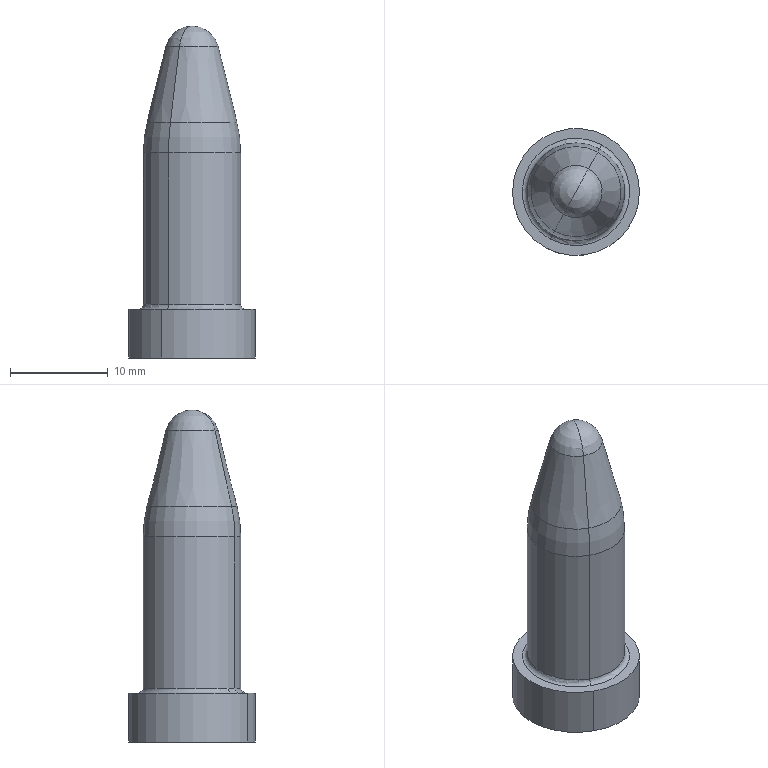Part | CATIA | 1 solid | 14 faces | box 13 x 13 x 34 mm | volume 2517 mm3 | cylinder 4 | torus 2 | other 2 | cone 2 | sphere 2 | plane 2 | commonest cylinder face diameters 10 x2 13 x2
STEP:
#1=CARTESIAN_POINT('',(3.116,5.704,-5.));
#2=VERTEX_POINT('',#1);
#3=CARTESIAN_POINT('',(-3.116,-5.704,-5.));
#4=VERTEX_POINT('',#3);
#5=CARTESIAN_POINT('',(0.,0.,-5.));
#6=DIRECTION('',(0.,0.,-1.));
#7=AXIS2_PLACEMENT_3D('',#5,#6,$);
#8=CIRCLE('',#7,6.5);
#9=EDGE_CURVE('',#2,#4,#8,.T.);
#10=ORIENTED_EDGE('',*,*,#9,.F.);
#11=CARTESIAN_POINT('',(3.116,5.704,0.));
#12=VERTEX_POINT('',#11);
#13=CARTESIAN_POINT('',(3.116,5.704,-2.5));
#14=DIRECTION('',(0.,0.,-1.));
#15=VECTOR('',#14,1.);
#16=LINE('',#13,#15);
#17=EDGE_CURVE('',#2,#12,#16,.F.);
#18=ORIENTED_EDGE('',*,*,#17,.T.);
#19=CARTESIAN_POINT('',(-3.116,-5.704,0.));
#20=VERTEX_POINT('',#19);
#21=CARTESIAN_POINT('',(0.,0.,0.));
#22=DIRECTION('',(0.,0.,-1.));
#23=AXIS2_PLACEMENT_3D('',#21,#22,$);
#24=CIRCLE('',#23,6.5);
#25=EDGE_CURVE('',#12,#20,#24,.T.);
#26=ORIENTED_EDGE('',*,*,#25,.T.);
#27=CARTESIAN_POINT('',(-3.116,-5.704,-2.5));
#28=DIRECTION('',(0.,0.,-1.));
#29=VECTOR('',#28,1.);
#30=LINE('',#27,#29);
#31=EDGE_CURVE('',#4,#20,#30,.F.);
#32=ORIENTED_EDGE('',*,*,#31,.F.);
#33=EDGE_LOOP('',(#10,#18,#26,#32));
#34=FACE_OUTER_BOUND('',#33,.T.);
#35=CARTESIAN_POINT('',(0.,0.,12.));
#36=DIRECTION('',(0.,0.,-1.));
#37=DIRECTION('',(0.4794,0.8776,0.));
#38=AXIS2_PLACEMENT_3D('',#35,#36,#37);
#39=CYLINDRICAL_SURFACE('',#38,6.5);
#40=ADVANCED_FACE('',(#34),#39,.T.);
#41=CARTESIAN_POINT('',(0.,0.,-5.));
#42=DIRECTION('',(0.,0.,-1.));
#43=AXIS2_PLACEMENT_3D('',#41,#42,$);
#44=CIRCLE('',#43,6.5);
#45=EDGE_CURVE('',#4,#2,#44,.T.);
#46=ORIENTED_EDGE('',*,*,#45,.F.);
#47=ORIENTED_EDGE('',*,*,#31,.T.);
#48=CARTESIAN_POINT('',(0.,0.,0.));
#49=DIRECTION('',(0.,0.,-1.));
#50=AXIS2_PLACEMENT_3D('',#48,#49,$);
#51=CIRCLE('',#50,6.5);
#52=EDGE_CURVE('',#20,#12,#51,.T.);
#53=ORIENTED_EDGE('',*,*,#52,.T.);
#54=ORIENTED_EDGE('',*,*,#17,.F.);
#55=EDGE_LOOP('',(#46,#47,#53,#54));
#56=FACE_OUTER_BOUND('',#55,.T.);
#57=ADVANCED_FACE('',(#56),#39,.T.);
#58=CARTESIAN_POINT('',(2.637,4.827,0.));
#59=VERTEX_POINT('',#58);
#60=CARTESIAN_POINT('',(-2.637,-4.827,0.));
#61=VERTEX_POINT('',#60);
#62=CARTESIAN_POINT('',(0.,0.,0.));
#63=DIRECTION('',(0.,0.,-1.));
#64=AXIS2_PLACEMENT_3D('',#62,#63,$);
#65=CIRCLE('',#64,5.5);
#66=EDGE_CURVE('',#59,#61,#65,.T.);
#67=ORIENTED_EDGE('',*,*,#66,.F.);
#68=CARTESIAN_POINT('',(2.397,4.388,0.5));
#69=VERTEX_POINT('',#68);
#70=CARTESIAN_POINT('',(2.637,4.827,0.5));
#71=DIRECTION('',(-0.8776,0.4794,0.));
#72=AXIS2_PLACEMENT_3D('',#70,#71,$);
#73=CIRCLE('',#72,0.5);
#74=EDGE_CURVE('',#59,#69,#73,.T.);
#75=ORIENTED_EDGE('',*,*,#74,.T.);
#76=CARTESIAN_POINT('',(-2.397,-4.388,0.5));
#77=VERTEX_POINT('',#76);
#78=CARTESIAN_POINT('',(0.,0.,0.5));
#79=DIRECTION('',(0.,0.,-1.));
#80=AXIS2_PLACEMENT_3D('',#78,#79,$);
#81=CIRCLE('',#80,5.);
#82=EDGE_CURVE('',#69,#77,#81,.T.);
#83=ORIENTED_EDGE('',*,*,#82,.T.);
#84=CARTESIAN_POINT('',(-2.637,-4.827,0.5));
#85=DIRECTION('',(0.8776,-0.4794,0.));
#86=AXIS2_PLACEMENT_3D('',#84,#85,$);
#87=CIRCLE('',#86,0.5);
#88=EDGE_CURVE('',#61,#77,#87,.T.);
#89=ORIENTED_EDGE('',*,*,#88,.F.);
#90=EDGE_LOOP('',(#67,#75,#83,#89));
#91=FACE_OUTER_BOUND('',#90,.T.);
#92=CARTESIAN_POINT('',(0.,0.,0.5));
#93=DIRECTION('',(0.,0.,-1.));
#94=DIRECTION('',(0.4794,0.8776,0.));
#95=AXIS2_PLACEMENT_3D('',#92,#93,#94);
#96=TOROIDAL_SURFACE('',#95,5.5,0.5);
#97=ADVANCED_FACE('',(#91),#96,.F.);
#98=CARTESIAN_POINT('',(0.,0.,0.));
#99=DIRECTION('',(0.,0.,-1.));
#100=AXIS2_PLACEMENT_3D('',#98,#99,$);
#101=CIRCLE('',#100,5.5);
#102=EDGE_CURVE('',#61,#59,#101,.T.);
#103=ORIENTED_EDGE('',*,*,#102,.F.);
#104=ORIENTED_EDGE('',*,*,#88,.T.);
#105=CARTESIAN_POINT('',(0.,0.,0.5));
#106=DIRECTION('',(0.,0.,-1.));
#107=AXIS2_PLACEMENT_3D('',#105,#106,$);
#108=CIRCLE('',#107,5.);
#109=EDGE_CURVE('',#77,#69,#108,.T.);
#110=ORIENTED_EDGE('',*,*,#109,.T.);
#111=ORIENTED_EDGE('',*,*,#74,.F.);
#112=EDGE_LOOP('',(#103,#104,#110,#111));
#113=FACE_OUTER_BOUND('',#112,.T.);
#114=ADVANCED_FACE('',(#113),#96,.F.);
#115=ORIENTED_EDGE('',*,*,#82,.F.);
#116=CARTESIAN_POINT('',(2.397,4.388,16.));
#117=VERTEX_POINT('',#116);
#118=CARTESIAN_POINT('',(2.397,4.388,8.25));
#119=DIRECTION('',(0.,0.,-1.));
#120=VECTOR('',#119,1.);
#121=LINE('',#118,#120);
#122=EDGE_CURVE('',#69,#117,#121,.F.);
#123=ORIENTED_EDGE('',*,*,#122,.T.);
#124=CARTESIAN_POINT('',(-2.397,-4.388,16.));
#125=VERTEX_POINT('',#124);
#126=CARTESIAN_POINT('',(0.,0.,16.));
#127=DIRECTION('',(0.,0.,-1.));
#128=AXIS2_PLACEMENT_3D('',#126,#127,$);
#129=CIRCLE('',#128,5.);
#130=EDGE_CURVE('',#117,#125,#129,.T.);
#131=ORIENTED_EDGE('',*,*,#130,.T.);
#132=CARTESIAN_POINT('',(-2.397,-4.388,8.25));
#133=DIRECTION('',(0.,0.,-1.));
#134=VECTOR('',#133,1.);
#135=LINE('',#132,#134);
#136=EDGE_CURVE('',#77,#125,#135,.F.);
#137=ORIENTED_EDGE('',*,*,#136,.F.);
#138=EDGE_LOOP('',(#115,#123,#131,#137));
#139=FACE_OUTER_BOUND('',#138,.T.);
#140=CARTESIAN_POINT('',(0.,0.,12.));
#141=DIRECTION('',(0.,0.,-1.));
#142=DIRECTION('',(0.4794,0.8776,0.));
#143=AXIS2_PLACEMENT_3D('',#140,#141,#142);
#144=CYLINDRICAL_SURFACE('',#143,5.);
#145=ADVANCED_FACE('',(#139),#144,.T.);
#146=ORIENTED_EDGE('',*,*,#109,.F.);
#147=ORIENTED_EDGE('',*,*,#136,.T.);
#148=CARTESIAN_POINT('',(0.,0.,16.));
#149=DIRECTION('',(0.,0.,-1.));
#150=AXIS2_PLACEMENT_3D('',#148,#149,$);
#151=CIRCLE('',#150,5.);
#152=EDGE_CURVE('',#125,#117,#151,.T.);
#153=ORIENTED_EDGE('',*,*,#152,.T.);
#154=ORIENTED_EDGE('',*,*,#122,.F.);
#155=EDGE_LOOP('',(#146,#147,#153,#154));
#156=FACE_OUTER_BOUND('',#155,.T.);
#157=ADVANCED_FACE('',(#156),#144,.T.);
#158=ORIENTED_EDGE('',*,*,#130,.F.);
#159=CARTESIAN_POINT('',(2.212,4.049,19.145));
#160=VERTEX_POINT('',#159);
#161=CARTESIAN_POINT('',(2.397,4.388,16.));
#162=CARTESIAN_POINT('',(2.397,4.388,17.059));
#163=CARTESIAN_POINT('',(2.335,4.274,18.118));
#164=CARTESIAN_POINT('',(2.212,4.049,19.145));
#165=B_SPLINE_CURVE_WITH_KNOTS('',3,(#161,#162,#163,#164),.UNSPECIFIED.,.F.,.U.,(4,4),(0.,3.176),.UNSPECIFIED.);
#166=EDGE_CURVE('',#117,#160,#165,.T.);
#167=ORIENTED_EDGE('',*,*,#166,.T.);
#168=CARTESIAN_POINT('',(-2.212,-4.049,19.145));
#169=VERTEX_POINT('',#168);
#170=CARTESIAN_POINT('',(0.,0.,19.145));
#171=DIRECTION('',(0.,0.,-1.));
#172=AXIS2_PLACEMENT_3D('',#170,#171,$);
#173=CIRCLE('',#172,4.614);
#174=EDGE_CURVE('',#160,#169,#173,.T.);
#175=ORIENTED_EDGE('',*,*,#174,.T.);
#176=CARTESIAN_POINT('',(-2.397,-4.388,16.));
#177=CARTESIAN_POINT('',(-2.397,-4.388,17.059));
#178=CARTESIAN_POINT('',(-2.335,-4.274,18.118));
#179=CARTESIAN_POINT('',(-2.212,-4.049,19.145));
#180=B_SPLINE_CURVE_WITH_KNOTS('',3,(#176,#177,#178,#179),.UNSPECIFIED.,.F.,.U.,(4,4),(0.,3.176),.UNSPECIFIED.);
#181=EDGE_CURVE('',#125,#169,#180,.T.);
#182=ORIENTED_EDGE('',*,*,#181,.F.);
#183=EDGE_LOOP('',(#158,#167,#175,#182));
#184=FACE_OUTER_BOUND('',#183,.T.);
#185=CARTESIAN_POINT('',(0.,5.,16.));
#186=CARTESIAN_POINT('',(0.,5.,17.059));
#187=CARTESIAN_POINT('',(0.,4.87,18.118));
#188=CARTESIAN_POINT('',(0.,4.614,19.145));
#189=B_SPLINE_CURVE_WITH_KNOTS('',3,(#185,#186,#187,#188),.UNSPECIFIED.,.F.,.U.,(4,4),(0.,3.176),.UNSPECIFIED.);
#190=CARTESIAN_POINT('',(0.,0.,12.));
#191=DIRECTION('',(0.,0.,-1.));
#192=AXIS1_PLACEMENT('',#190,#191);
#193=SURFACE_OF_REVOLUTION('',#189,#192);
#194=ADVANCED_FACE('',(#184),#193,.F.);
#195=ORIENTED_EDGE('',*,*,#152,.F.);
#196=ORIENTED_EDGE('',*,*,#181,.T.);
#197=CARTESIAN_POINT('',(0.,0.,19.145));
#198=DIRECTION('',(0.,0.,-1.));
#199=AXIS2_PLACEMENT_3D('',#197,#198,$);
#200=CIRCLE('',#199,4.614);
#201=EDGE_CURVE('',#169,#160,#200,.T.);
#202=ORIENTED_EDGE('',*,*,#201,.T.);
#203=ORIENTED_EDGE('',*,*,#166,.F.);
#204=EDGE_LOOP('',(#195,#196,#202,#203));
#205=FACE_OUTER_BOUND('',#204,.T.);
#206=CARTESIAN_POINT('',(0.,5.,16.));
#207=CARTESIAN_POINT('',(0.,5.,17.059));
#208=CARTESIAN_POINT('',(0.,4.87,18.118));
#209=CARTESIAN_POINT('',(0.,4.614,19.145));
#210=B_SPLINE_CURVE_WITH_KNOTS('',3,(#206,#207,#208,#209),.UNSPECIFIED.,.F.,.U.,(4,4),(0.,3.176),.UNSPECIFIED.);
#211=CARTESIAN_POINT('',(0.,0.,12.));
#212=DIRECTION('',(0.,0.,-1.));
#213=AXIS1_PLACEMENT('',#211,#212);
#214=SURFACE_OF_REVOLUTION('',#210,#213);
#215=ADVANCED_FACE('',(#205),#214,.F.);
#216=ORIENTED_EDGE('',*,*,#174,.F.);
#217=CARTESIAN_POINT('',(1.284,2.351,26.907));
#218=VERTEX_POINT('',#217);
#219=CARTESIAN_POINT('',(1.748,3.2,23.026));
#220=DIRECTION('',(0.116,0.2123,-0.9703));
#221=VECTOR('',#220,1.);
#222=LINE('',#219,#221);
#223=EDGE_CURVE('',#160,#218,#222,.F.);
#224=ORIENTED_EDGE('',*,*,#223,.T.);
#225=CARTESIAN_POINT('',(-1.284,-2.351,26.907));
#226=VERTEX_POINT('',#225);
#227=CARTESIAN_POINT('',(0.,0.,26.907));
#228=DIRECTION('',(0.,0.,-1.));
#229=AXIS2_PLACEMENT_3D('',#227,#228,$);
#230=CIRCLE('',#229,2.678);
#231=EDGE_CURVE('',#218,#226,#230,.T.);
#232=ORIENTED_EDGE('',*,*,#231,.T.);
#233=CARTESIAN_POINT('',(-1.748,-3.2,23.026));
#234=DIRECTION('',(-0.116,-0.2123,-0.9703));
#235=VECTOR('',#234,1.);
#236=LINE('',#233,#235);
#237=EDGE_CURVE('',#169,#226,#236,.F.);
#238=ORIENTED_EDGE('',*,*,#237,.F.);
#239=EDGE_LOOP('',(#216,#224,#232,#238));
#240=FACE_OUTER_BOUND('',#239,.T.);
#241=CARTESIAN_POINT('',(0.,0.,26.907));
#242=DIRECTION('',(0.,0.,-1.));
#243=DIRECTION('',(0.4794,0.8776,0.));
#244=AXIS2_PLACEMENT_3D('',#241,#242,#243);
#245=CONICAL_SURFACE('',#244,2.678,0.2443);
#246=ADVANCED_FACE('',(#240),#245,.T.);
#247=ORIENTED_EDGE('',*,*,#201,.F.);
#248=ORIENTED_EDGE('',*,*,#237,.T.);
#249=CARTESIAN_POINT('',(0.,0.,26.907));
#250=DIRECTION('',(0.,0.,-1.));
#251=AXIS2_PLACEMENT_3D('',#249,#250,$);
#252=CIRCLE('',#251,2.678);
#253=EDGE_CURVE('',#226,#218,#252,.T.);
#254=ORIENTED_EDGE('',*,*,#253,.T.);
#255=ORIENTED_EDGE('',*,*,#223,.F.);
#256=EDGE_LOOP('',(#247,#248,#254,#255));
#257=FACE_OUTER_BOUND('',#256,.T.);
#258=ADVANCED_FACE('',(#257),#245,.T.);
#259=ORIENTED_EDGE('',*,*,#231,.F.);
#260=CARTESIAN_POINT('',(0.,0.,29.));
#261=VERTEX_POINT('',#260);
#262=CARTESIAN_POINT('',(0.,0.,26.24));
#263=DIRECTION('',(-0.8776,0.4794,0.));
#264=AXIS2_PLACEMENT_3D('',#262,#263,$);
#265=CIRCLE('',#264,2.76);
#266=EDGE_CURVE('',#218,#261,#265,.F.);
#267=ORIENTED_EDGE('',*,*,#266,.T.);
#268=CARTESIAN_POINT('',(0.,0.,26.24));
#269=DIRECTION('',(0.8776,-0.4794,0.));
#270=AXIS2_PLACEMENT_3D('',#268,#269,$);
#271=CIRCLE('',#270,2.76);
#272=EDGE_CURVE('',#226,#261,#271,.F.);
#273=ORIENTED_EDGE('',*,*,#272,.F.);
#274=EDGE_LOOP('',(#259,#267,#273));
#275=FACE_OUTER_BOUND('',#274,.T.);
#276=CARTESIAN_POINT('',(0.,0.,26.24));
#277=DIRECTION('',(0.,0.,-1.));
#278=DIRECTION('',(0.4794,0.8776,0.));
#279=AXIS2_PLACEMENT_3D('',#276,#277,#278);
#280=SPHERICAL_SURFACE('',#279,2.76);
#281=ADVANCED_FACE('',(#275),#280,.T.);
#282=ORIENTED_EDGE('',*,*,#253,.F.);
#283=ORIENTED_EDGE('',*,*,#272,.T.);
#284=ORIENTED_EDGE('',*,*,#266,.F.);
#285=EDGE_LOOP('',(#282,#283,#284));
#286=FACE_OUTER_BOUND('',#285,.T.);
#287=ADVANCED_FACE('',(#286),#280,.T.);
#288=ORIENTED_EDGE('',*,*,#9,.T.);
#289=ORIENTED_EDGE('',*,*,#45,.T.);
#290=EDGE_LOOP('',(#288,#289));
#291=FACE_OUTER_BOUND('',#290,.T.);
#292=CARTESIAN_POINT('',(0.,0.,-5.));
#293=DIRECTION('',(0.,0.,-1.));
#294=DIRECTION('',(1.,0.,0.));
#295=AXIS2_PLACEMENT_3D('',#292,#293,#294);
#296=PLANE('',#295);
#297=ADVANCED_FACE('',(#291),#296,.T.);
#298=ORIENTED_EDGE('',*,*,#25,.F.);
#299=ORIENTED_EDGE('',*,*,#52,.F.);
#300=EDGE_LOOP('',(#298,#299));
#301=FACE_OUTER_BOUND('',#300,.T.);
#302=ORIENTED_EDGE('',*,*,#102,.T.);
#303=ORIENTED_EDGE('',*,*,#66,.T.);
#304=EDGE_LOOP('',(#302,#303));
#305=FACE_BOUND('',#304,.T.);
#306=CARTESIAN_POINT('',(0.,6.5,0.));
#307=DIRECTION('',(0.,0.,-1.));
#308=DIRECTION('',(1.,0.,0.));
#309=AXIS2_PLACEMENT_3D('',#306,#307,#308);
#310=PLANE('',#309);
#311=ADVANCED_FACE('',(#301,#305),#310,.F.);
#312=CLOSED_SHELL('',(#40,#57,#97,#114,#145,#157,#194,#215,#246,#258,#281,#287,#297,#311));
#313=MANIFOLD_SOLID_BREP('',#312);
#314=(LENGTH_UNIT()NAMED_UNIT(*)SI_UNIT(.MILLI.,.METRE.));
#315=UNCERTAINTY_MEASURE_WITH_UNIT(LENGTH_MEASURE(0.005),#314,'','');
#316=(NAMED_UNIT(*)PLANE_ANGLE_UNIT()SI_UNIT($,.RADIAN.));
#317=(NAMED_UNIT(*)SI_UNIT($,.STERADIAN.)SOLID_ANGLE_UNIT());
#318=(GEOMETRIC_REPRESENTATION_CONTEXT(3)GLOBAL_UNCERTAINTY_ASSIGNED_CONTEXT((#315))GLOBAL_UNIT_ASSIGNED_CONTEXT((#314,#316,#317))REPRESENTATION_CONTEXT('',''));
#319=ADVANCED_BREP_SHAPE_REPRESENTATION('',(#313),#318);